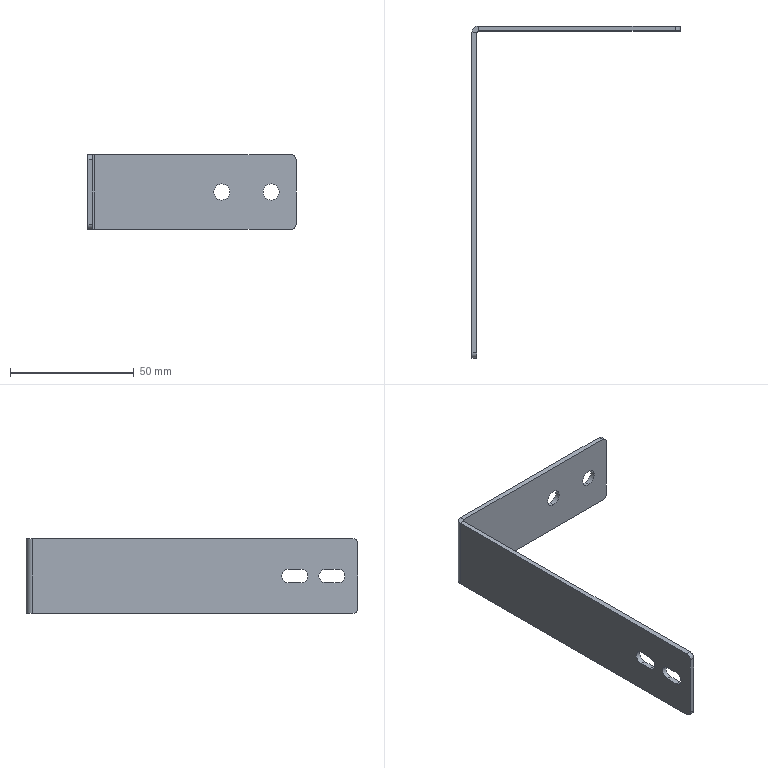Part | STEP file | PN_0032 | 1 solid | 32 faces | box 84 x 134 x 30 mm | volume 12571 mm3 | cylinder 16 | plane 16 | commonest cylinder face diameters 5.5 x6 4 x4 6.5 x4 1.473 x1 5.473 x1